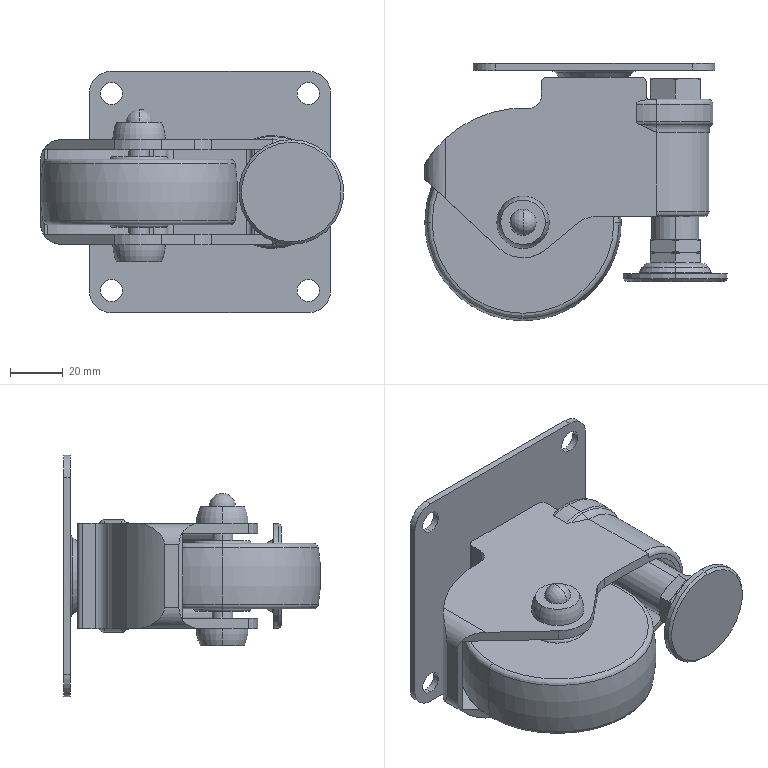Part | SolidWorks | features AEMSimFeature 1 | 4 solids | 212 faces | box 115.5 x 98 x 92 mm | volume 222779 mm3 | plane 71 | cylinder 54 | cone 47 | torus 38 | sphere 2 | commonest cylinder face diameters 8.5 x8 17 x6 4 x5 8 x4 12 x4 20 x4